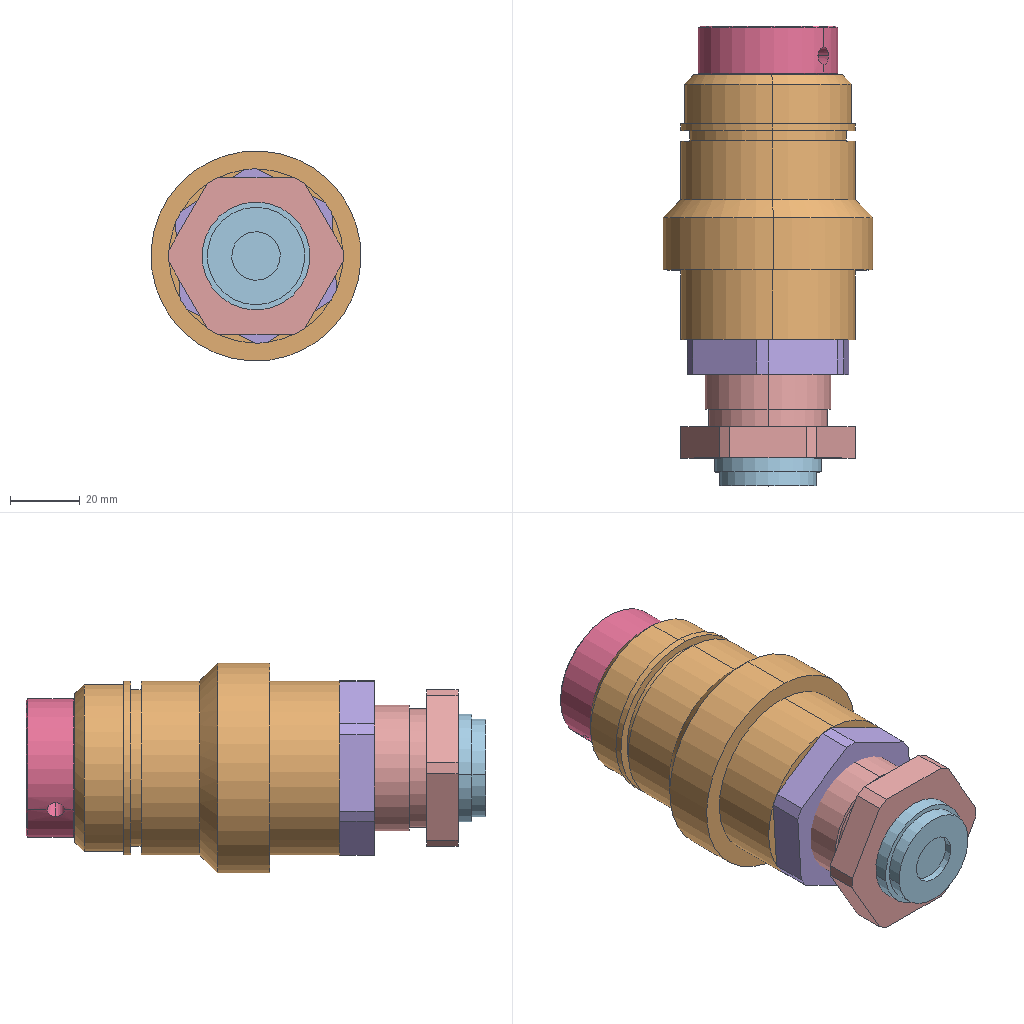Assembly | SolidWorks | 10 different items | 10 placed | box 60 x 132 x 60 mm
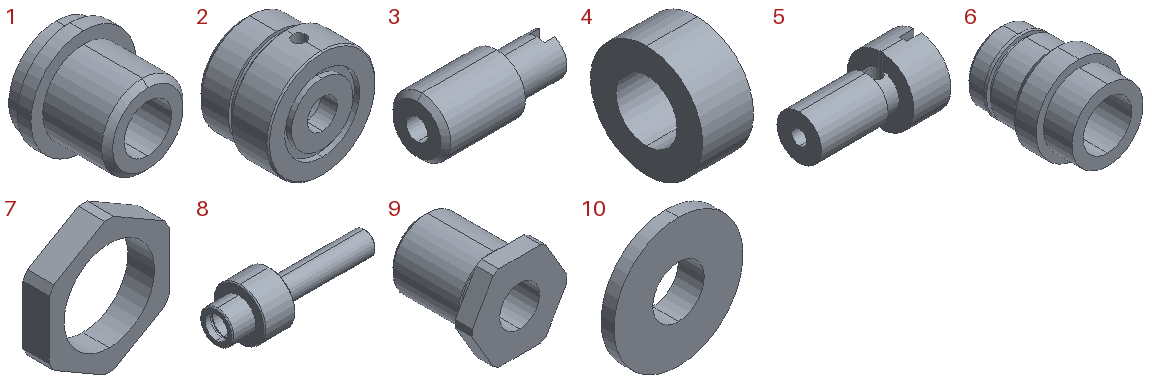Parts list (item | quantity | size | volume | features):
1 | x1 | 31 x 27 x 31 mm | 11981 mm3 | features ICE 4, Extrusion 1, StudWizard 1
2 | x1 | 40 x 29 x 40 mm | 19721 mm3 | features ICE 6, Chamfer 1, Extrusion 1, StudWizard 1
3 | x1 | 18 x 8 x 8 mm | 579.241 mm3 | features ICE 3, Extrusion 1, StudWizard 1
4 | x1 | 5 x 11 x 11 mm | 333.794 mm3 | features Extrusion 1
5 | x1 | 16 x 9 x 9 mm | 549.177 mm3 | features ICE 5, Extrusion 1
6 | x1 | 60.3 x 76 x 60.3 mm | 93894 mm3 | features ICE 7, HoleWzd 2, Chamfer 1, Extrusion 1, StudWizard 1
7 | x1 | 45 x 10 x 50 mm | 8358 mm3 | features CirPattern 1, Extrusion 1, HoleWzd 1, ICE 1
8 | x1 | 72 x 25 x 25 mm | 11483 mm3 | features ICE 9, Chamfer 1, Extrusion 1, HoleWzd 1
9 | x1 | 50 x 53 x 45 mm | 40001 mm3 | features ICE 8, Chamfer 1, Extrusion 1, HoleWzd 1, StudWizard 1
10 | x1 | 30 x 6 x 30 mm | 2293 mm3 | features ICE 2, Extrusion 1
Mates (type | each side: item.copy, entity, surface, feature):
Concentric | 9.1 face cylinder M36 Mechanical Thread Stud1 | 6.1 face cylinder Boss-Extrude5
Concentric | 6.1 face cylinder Boss-Extrude1 | 8.1 face cylinder Boss-Extrude3
Concentric | 3.1 face cylinder Boss-Extrude2 | 6.1 face cylinder Boss-Extrude1
Concentric | 5.1 face cylinder Boss-Extrude3 | 6.1 face cylinder Boss-Extrude1
Concentric | 4.1 face cylinder Boss-Extrude1 | 6.1 face cylinder Boss-Extrude1
Concentric | 9.1 face cylinder M36 Mechanical Thread Stud1 | 7.1 face cylinder M36x2.0 Tapped Hole1
Concentric | 10.1 face cylinder Cut-Extrude1 | 8.1 face cylinder Boss-Extrude1
Coincident | 10.1 face plane Boss-Extrude1 | 8.1 face plane Boss-Extrude2
Coincident | 3.1 face plane Boss-Extrude1 | 8.1 face plane Boss-Extrude4
Coincident | 4.1 face plane Boss-Extrude1 | 5.1 face plane Boss-Extrude3
Coincident | 5.1 face plane Boss-Extrude3 | 8.1 face plane Cut-Extrude3
Coincident | 6.1 face plane Boss-Extrude1 | 7.1 face plane Boss-Extrude1
Concentric | 9.1 face cylinder M24 Tapped Hole1 | 1.1 face cylinder M24 Mechanical Thread Stud1
Coincident | 9.1 face plane Boss-Extrude1 | 1.1 face plane Boss-Extrude2
Concentric | 6.1 face cylinder Boss-Extrude1 | 2.1 face cylinder Boss-Extrude1
Coincident | 6.1 face plane Boss-Extrude4 | 2.1 face plane Boss-Extrude1
Coincident | 8.1 face plane Boss-Extrude1 | 2.1 face plane Cut-Extrude1
DistanceDim | 7.1 face plane Boss-Extrude1 | 9.1 face plane Boss-Extrude3